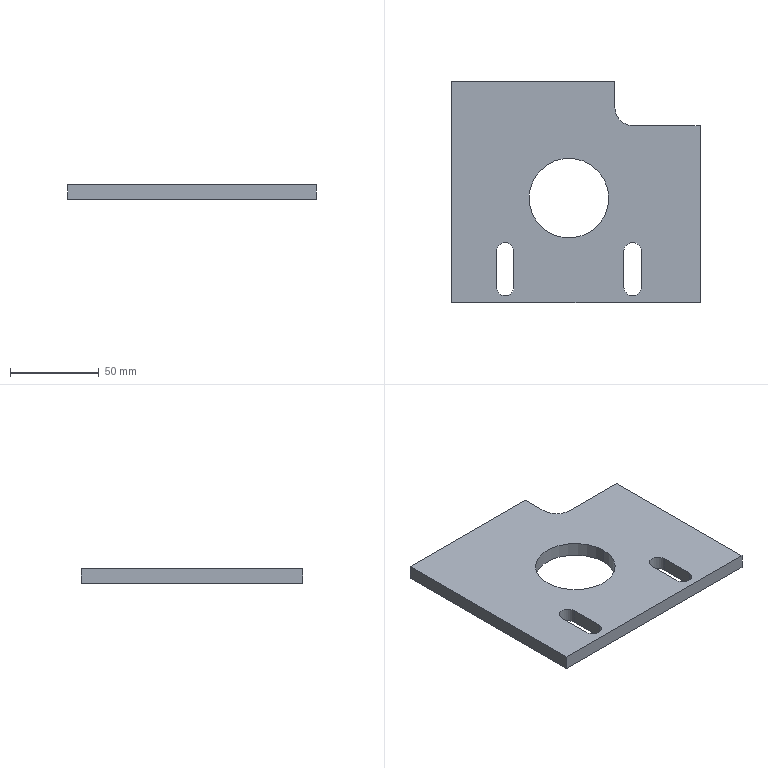Part | SolidWorks | features ICE 3, Extrusion 1, Fillet 1, LPattern 1 | 1 solid | 19 faces | box 140 x 125 x 8 mm | volume 113392 mm3 | plane 12 | cylinder 7 | commonest cylinder face diameters 10 x4 45 x2 20 x1
STEP:
#1=CARTESIAN_POINT('',(43.5,-66.,0.));
#2=VERTEX_POINT('',#1);
#3=CARTESIAN_POINT('',(88.5,-66.,0.));
#4=VERTEX_POINT('',#3);
#5=CARTESIAN_POINT('',(66.,-66.,0.));
#6=DIRECTION('',(0.,0.,1.));
#7=DIRECTION('',(1.,0.,0.));
#8=AXIS2_PLACEMENT_3D('',#5,#6,#7);
#9=CIRCLE('',#8,22.5);
#10=EDGE_CURVE('',#2,#4,#9,.T.);
#11=ORIENTED_EDGE('',*,*,#10,.F.);
#12=CARTESIAN_POINT('',(43.5,-66.,8.));
#13=VERTEX_POINT('',#12);
#14=CARTESIAN_POINT('',(43.5,-66.,0.));
#15=DIRECTION('',(0.,0.,1.));
#16=VECTOR('',#15,1000.);
#17=LINE('',#14,#16);
#18=EDGE_CURVE('',#2,#13,#17,.T.);
#19=ORIENTED_EDGE('',*,*,#18,.T.);
#20=CARTESIAN_POINT('',(88.5,-66.,8.));
#21=VERTEX_POINT('',#20);
#22=CARTESIAN_POINT('',(66.,-66.,8.));
#23=DIRECTION('',(0.,0.,1.));
#24=DIRECTION('',(1.,0.,0.));
#25=AXIS2_PLACEMENT_3D('',#22,#23,#24);
#26=CIRCLE('',#25,22.5);
#27=EDGE_CURVE('',#13,#21,#26,.T.);
#28=ORIENTED_EDGE('',*,*,#27,.T.);
#29=CARTESIAN_POINT('',(88.5,-66.,0.));
#30=DIRECTION('',(0.,0.,1.));
#31=VECTOR('',#30,1000.);
#32=LINE('',#29,#31);
#33=EDGE_CURVE('',#4,#21,#32,.T.);
#34=ORIENTED_EDGE('',*,*,#33,.F.);
#35=EDGE_LOOP('',(#11,#19,#28,#34));
#36=FACE_OUTER_BOUND('',#35,.T.);
#37=CARTESIAN_POINT('',(66.,-66.,0.));
#38=DIRECTION('',(0.,0.,1.));
#39=DIRECTION('',(1.,0.,0.));
#40=AXIS2_PLACEMENT_3D('',#37,#38,#39);
#41=CYLINDRICAL_SURFACE('',#40,22.5);
#42=ADVANCED_FACE('',(#36),#41,.F.);
#43=CARTESIAN_POINT('',(0.,0.,0.));
#44=VERTEX_POINT('',#43);
#45=CARTESIAN_POINT('',(0.,-125.,0.));
#46=VERTEX_POINT('',#45);
#47=CARTESIAN_POINT('',(0.,0.,0.));
#48=DIRECTION('',(0.,-1.,0.));
#49=VECTOR('',#48,1000.);
#50=LINE('',#47,#49);
#51=EDGE_CURVE('',#44,#46,#50,.T.);
#52=ORIENTED_EDGE('',*,*,#51,.T.);
#53=CARTESIAN_POINT('',(0.,-125.,8.));
#54=VERTEX_POINT('',#53);
#55=CARTESIAN_POINT('',(0.,-125.,8.));
#56=DIRECTION('',(0.,0.,-1.));
#57=VECTOR('',#56,1000.);
#58=LINE('',#55,#57);
#59=EDGE_CURVE('',#54,#46,#58,.T.);
#60=ORIENTED_EDGE('',*,*,#59,.F.);
#61=CARTESIAN_POINT('',(0.,0.,8.));
#62=VERTEX_POINT('',#61);
#63=CARTESIAN_POINT('',(0.,0.,8.));
#64=DIRECTION('',(0.,-1.,0.));
#65=VECTOR('',#64,1000.);
#66=LINE('',#63,#65);
#67=EDGE_CURVE('',#62,#54,#66,.T.);
#68=ORIENTED_EDGE('',*,*,#67,.F.);
#69=CARTESIAN_POINT('',(0.,0.,8.));
#70=DIRECTION('',(0.,0.,-1.));
#71=VECTOR('',#70,1000.);
#72=LINE('',#69,#71);
#73=EDGE_CURVE('',#62,#44,#72,.T.);
#74=ORIENTED_EDGE('',*,*,#73,.T.);
#75=EDGE_LOOP('',(#52,#60,#68,#74));
#76=FACE_OUTER_BOUND('',#75,.T.);
#77=CARTESIAN_POINT('',(0.,0.,8.));
#78=DIRECTION('',(1.,0.,0.));
#79=DIRECTION('',(0.,0.,-1.));
#80=AXIS2_PLACEMENT_3D('',#77,#78,#79);
#81=PLANE('',#80);
#82=ADVANCED_FACE('',(#76),#81,.F.);
#83=CARTESIAN_POINT('',(140.,-125.,0.));
#84=VERTEX_POINT('',#83);
#85=CARTESIAN_POINT('',(0.,-125.,0.));
#86=DIRECTION('',(1.,0.,0.));
#87=VECTOR('',#86,1000.);
#88=LINE('',#85,#87);
#89=EDGE_CURVE('',#46,#84,#88,.T.);
#90=ORIENTED_EDGE('',*,*,#89,.T.);
#91=CARTESIAN_POINT('',(140.,-125.,8.));
#92=VERTEX_POINT('',#91);
#93=CARTESIAN_POINT('',(140.,-125.,8.));
#94=DIRECTION('',(0.,0.,-1.));
#95=VECTOR('',#94,1000.);
#96=LINE('',#93,#95);
#97=EDGE_CURVE('',#92,#84,#96,.T.);
#98=ORIENTED_EDGE('',*,*,#97,.F.);
#99=CARTESIAN_POINT('',(0.,-125.,8.));
#100=DIRECTION('',(1.,0.,0.));
#101=VECTOR('',#100,1000.);
#102=LINE('',#99,#101);
#103=EDGE_CURVE('',#54,#92,#102,.T.);
#104=ORIENTED_EDGE('',*,*,#103,.F.);
#105=ORIENTED_EDGE('',*,*,#59,.T.);
#106=EDGE_LOOP('',(#90,#98,#104,#105));
#107=FACE_OUTER_BOUND('',#106,.T.);
#108=CARTESIAN_POINT('',(0.,-125.,8.));
#109=DIRECTION('',(0.,1.,0.));
#110=DIRECTION('',(0.,0.,1.));
#111=AXIS2_PLACEMENT_3D('',#108,#109,#110);
#112=PLANE('',#111);
#113=ADVANCED_FACE('',(#107),#112,.F.);
#114=CARTESIAN_POINT('',(140.,-25.,0.));
#115=VERTEX_POINT('',#114);
#116=CARTESIAN_POINT('',(140.,0.,0.));
#117=DIRECTION('',(0.,1.,0.));
#118=VECTOR('',#117,1000.);
#119=LINE('',#116,#118);
#120=EDGE_CURVE('',#84,#115,#119,.T.);
#121=ORIENTED_EDGE('',*,*,#120,.T.);
#122=CARTESIAN_POINT('',(140.,-25.,8.));
#123=VERTEX_POINT('',#122);
#124=CARTESIAN_POINT('',(140.,-25.,0.));
#125=DIRECTION('',(0.,0.,1.));
#126=VECTOR('',#125,1000.);
#127=LINE('',#124,#126);
#128=EDGE_CURVE('',#115,#123,#127,.T.);
#129=ORIENTED_EDGE('',*,*,#128,.T.);
#130=CARTESIAN_POINT('',(140.,0.,8.));
#131=DIRECTION('',(0.,1.,0.));
#132=VECTOR('',#131,1000.);
#133=LINE('',#130,#132);
#134=EDGE_CURVE('',#92,#123,#133,.T.);
#135=ORIENTED_EDGE('',*,*,#134,.F.);
#136=ORIENTED_EDGE('',*,*,#97,.T.);
#137=EDGE_LOOP('',(#121,#129,#135,#136));
#138=FACE_OUTER_BOUND('',#137,.T.);
#139=CARTESIAN_POINT('',(140.,0.,8.));
#140=DIRECTION('',(-1.,0.,0.));
#141=DIRECTION('',(0.,-1.,0.));
#142=AXIS2_PLACEMENT_3D('',#139,#140,#141);
#143=PLANE('',#142);
#144=ADVANCED_FACE('',(#138),#143,.F.);
#145=CARTESIAN_POINT('',(92.,0.,8.));
#146=VERTEX_POINT('',#145);
#147=CARTESIAN_POINT('',(0.,0.,8.));
#148=DIRECTION('',(-1.,0.,0.));
#149=VECTOR('',#148,1000.);
#150=LINE('',#147,#149);
#151=EDGE_CURVE('',#146,#62,#150,.T.);
#152=ORIENTED_EDGE('',*,*,#151,.F.);
#153=CARTESIAN_POINT('',(92.,0.,0.));
#154=VERTEX_POINT('',#153);
#155=CARTESIAN_POINT('',(92.,0.,0.));
#156=DIRECTION('',(0.,0.,1.));
#157=VECTOR('',#156,1000.);
#158=LINE('',#155,#157);
#159=EDGE_CURVE('',#154,#146,#158,.T.);
#160=ORIENTED_EDGE('',*,*,#159,.F.);
#161=CARTESIAN_POINT('',(0.,0.,0.));
#162=DIRECTION('',(-1.,0.,0.));
#163=VECTOR('',#162,1000.);
#164=LINE('',#161,#163);
#165=EDGE_CURVE('',#154,#44,#164,.T.);
#166=ORIENTED_EDGE('',*,*,#165,.T.);
#167=ORIENTED_EDGE('',*,*,#73,.F.);
#168=EDGE_LOOP('',(#152,#160,#166,#167));
#169=FACE_OUTER_BOUND('',#168,.T.);
#170=CARTESIAN_POINT('',(0.,0.,8.));
#171=DIRECTION('',(0.,-1.,0.));
#172=DIRECTION('',(0.,0.,-1.));
#173=AXIS2_PLACEMENT_3D('',#170,#171,#172);
#174=PLANE('',#173);
#175=ADVANCED_FACE('',(#169),#174,.F.);
#176=CARTESIAN_POINT('',(92.,-15.,8.));
#177=VERTEX_POINT('',#176);
#178=CARTESIAN_POINT('',(92.,0.,8.));
#179=DIRECTION('',(0.,-1.,0.));
#180=VECTOR('',#179,1000.);
#181=LINE('',#178,#180);
#182=EDGE_CURVE('',#146,#177,#181,.T.);
#183=ORIENTED_EDGE('',*,*,#182,.F.);
#184=ORIENTED_EDGE('',*,*,#151,.T.);
#185=ORIENTED_EDGE('',*,*,#67,.T.);
#186=ORIENTED_EDGE('',*,*,#103,.T.);
#187=ORIENTED_EDGE('',*,*,#134,.T.);
#188=CARTESIAN_POINT('',(102.,-25.,8.));
#189=VERTEX_POINT('',#188);
#190=CARTESIAN_POINT('',(92.,-25.,8.));
#191=DIRECTION('',(1.,0.,0.));
#192=VECTOR('',#191,1000.);
#193=LINE('',#190,#192);
#194=EDGE_CURVE('',#189,#123,#193,.T.);
#195=ORIENTED_EDGE('',*,*,#194,.F.);
#196=CARTESIAN_POINT('',(102.,-15.,8.));
#197=DIRECTION('',(0.,0.,-1.));
#198=DIRECTION('',(1.,0.,0.));
#199=AXIS2_PLACEMENT_3D('',#196,#197,#198);
#200=CIRCLE('',#199,10.);
#201=EDGE_CURVE('',#189,#177,#200,.T.);
#202=ORIENTED_EDGE('',*,*,#201,.T.);
#203=EDGE_LOOP('',(#183,#184,#185,#186,#187,#195,#202));
#204=FACE_OUTER_BOUND('',#203,.T.);
#205=CARTESIAN_POINT('',(107.,-96.,8.));
#206=VERTEX_POINT('',#205);
#207=CARTESIAN_POINT('',(97.,-96.,8.));
#208=VERTEX_POINT('',#207);
#209=CARTESIAN_POINT('',(102.,-96.,8.));
#210=DIRECTION('',(0.,0.,1.));
#211=DIRECTION('',(1.,0.,0.));
#212=AXIS2_PLACEMENT_3D('',#209,#210,#211);
#213=CIRCLE('',#212,5.);
#214=EDGE_CURVE('',#206,#208,#213,.T.);
#215=ORIENTED_EDGE('',*,*,#214,.F.);
#216=CARTESIAN_POINT('',(107.,-116.,8.));
#217=VERTEX_POINT('',#216);
#218=CARTESIAN_POINT('',(107.,-96.,8.));
#219=DIRECTION('',(0.,1.,0.));
#220=VECTOR('',#219,1000.);
#221=LINE('',#218,#220);
#222=EDGE_CURVE('',#217,#206,#221,.T.);
#223=ORIENTED_EDGE('',*,*,#222,.F.);
#224=CARTESIAN_POINT('',(97.,-116.,8.));
#225=VERTEX_POINT('',#224);
#226=CARTESIAN_POINT('',(102.,-116.,8.));
#227=DIRECTION('',(0.,0.,1.));
#228=DIRECTION('',(1.,0.,0.));
#229=AXIS2_PLACEMENT_3D('',#226,#227,#228);
#230=CIRCLE('',#229,5.);
#231=EDGE_CURVE('',#225,#217,#230,.T.);
#232=ORIENTED_EDGE('',*,*,#231,.F.);
#233=CARTESIAN_POINT('',(97.,-96.,8.));
#234=DIRECTION('',(0.,-1.,0.));
#235=VECTOR('',#234,1000.);
#236=LINE('',#233,#235);
#237=EDGE_CURVE('',#208,#225,#236,.T.);
#238=ORIENTED_EDGE('',*,*,#237,.F.);
#239=EDGE_LOOP('',(#215,#223,#232,#238));
#240=FACE_BOUND('',#239,.T.);
#241=CARTESIAN_POINT('',(35.,-96.,8.));
#242=VERTEX_POINT('',#241);
#243=CARTESIAN_POINT('',(25.,-96.,8.));
#244=VERTEX_POINT('',#243);
#245=CARTESIAN_POINT('',(30.,-96.,8.));
#246=DIRECTION('',(0.,0.,1.));
#247=DIRECTION('',(1.,0.,0.));
#248=AXIS2_PLACEMENT_3D('',#245,#246,#247);
#249=CIRCLE('',#248,5.);
#250=EDGE_CURVE('',#242,#244,#249,.T.);
#251=ORIENTED_EDGE('',*,*,#250,.F.);
#252=CARTESIAN_POINT('',(35.,-116.,8.));
#253=VERTEX_POINT('',#252);
#254=CARTESIAN_POINT('',(35.,-96.,8.));
#255=DIRECTION('',(0.,1.,0.));
#256=VECTOR('',#255,1000.);
#257=LINE('',#254,#256);
#258=EDGE_CURVE('',#253,#242,#257,.T.);
#259=ORIENTED_EDGE('',*,*,#258,.F.);
#260=CARTESIAN_POINT('',(25.,-116.,8.));
#261=VERTEX_POINT('',#260);
#262=CARTESIAN_POINT('',(30.,-116.,8.));
#263=DIRECTION('',(0.,0.,1.));
#264=DIRECTION('',(1.,0.,0.));
#265=AXIS2_PLACEMENT_3D('',#262,#263,#264);
#266=CIRCLE('',#265,5.);
#267=EDGE_CURVE('',#261,#253,#266,.T.);
#268=ORIENTED_EDGE('',*,*,#267,.F.);
#269=CARTESIAN_POINT('',(25.,-96.,8.));
#270=DIRECTION('',(0.,-1.,0.));
#271=VECTOR('',#270,1000.);
#272=LINE('',#269,#271);
#273=EDGE_CURVE('',#244,#261,#272,.T.);
#274=ORIENTED_EDGE('',*,*,#273,.F.);
#275=EDGE_LOOP('',(#251,#259,#268,#274));
#276=FACE_BOUND('',#275,.T.);
#277=CARTESIAN_POINT('',(66.,-66.,8.));
#278=DIRECTION('',(0.,0.,1.));
#279=DIRECTION('',(1.,0.,0.));
#280=AXIS2_PLACEMENT_3D('',#277,#278,#279);
#281=CIRCLE('',#280,22.5);
#282=EDGE_CURVE('',#21,#13,#281,.T.);
#283=ORIENTED_EDGE('',*,*,#282,.F.);
#284=ORIENTED_EDGE('',*,*,#27,.F.);
#285=EDGE_LOOP('',(#283,#284));
#286=FACE_BOUND('',#285,.T.);
#287=CARTESIAN_POINT('',(0.,0.,8.));
#288=DIRECTION('',(0.,0.,1.));
#289=DIRECTION('',(1.,0.,0.));
#290=AXIS2_PLACEMENT_3D('',#287,#288,#289);
#291=PLANE('',#290);
#292=ADVANCED_FACE('',(#204,#240,#276,#286),#291,.T.);
#293=CARTESIAN_POINT('',(107.,-116.,0.));
#294=VERTEX_POINT('',#293);
#295=CARTESIAN_POINT('',(107.,-96.,0.));
#296=VERTEX_POINT('',#295);
#297=CARTESIAN_POINT('',(107.,-96.,0.));
#298=DIRECTION('',(0.,1.,0.));
#299=VECTOR('',#298,1000.);
#300=LINE('',#297,#299);
#301=EDGE_CURVE('',#294,#296,#300,.T.);
#302=ORIENTED_EDGE('',*,*,#301,.T.);
#303=CARTESIAN_POINT('',(97.,-96.,0.));
#304=VERTEX_POINT('',#303);
#305=CARTESIAN_POINT('',(102.,-96.,0.));
#306=DIRECTION('',(0.,0.,1.));
#307=DIRECTION('',(1.,0.,0.));
#308=AXIS2_PLACEMENT_3D('',#305,#306,#307);
#309=CIRCLE('',#308,5.);
#310=EDGE_CURVE('',#296,#304,#309,.T.);
#311=ORIENTED_EDGE('',*,*,#310,.T.);
#312=CARTESIAN_POINT('',(97.,-116.,0.));
#313=VERTEX_POINT('',#312);
#314=CARTESIAN_POINT('',(97.,-96.,0.));
#315=DIRECTION('',(0.,-1.,0.));
#316=VECTOR('',#315,1000.);
#317=LINE('',#314,#316);
#318=EDGE_CURVE('',#304,#313,#317,.T.);
#319=ORIENTED_EDGE('',*,*,#318,.T.);
#320=CARTESIAN_POINT('',(102.,-116.,0.));
#321=DIRECTION('',(0.,0.,1.));
#322=DIRECTION('',(1.,0.,0.));
#323=AXIS2_PLACEMENT_3D('',#320,#321,#322);
#324=CIRCLE('',#323,5.);
#325=EDGE_CURVE('',#313,#294,#324,.T.);
#326=ORIENTED_EDGE('',*,*,#325,.T.);
#327=EDGE_LOOP('',(#302,#311,#319,#326));
#328=FACE_BOUND('',#327,.T.);
#329=CARTESIAN_POINT('',(35.,-116.,0.));
#330=VERTEX_POINT('',#329);
#331=CARTESIAN_POINT('',(35.,-96.,0.));
#332=VERTEX_POINT('',#331);
#333=CARTESIAN_POINT('',(35.,-96.,0.));
#334=DIRECTION('',(0.,1.,0.));
#335=VECTOR('',#334,1000.);
#336=LINE('',#333,#335);
#337=EDGE_CURVE('',#330,#332,#336,.T.);
#338=ORIENTED_EDGE('',*,*,#337,.T.);
#339=CARTESIAN_POINT('',(25.,-96.,0.));
#340=VERTEX_POINT('',#339);
#341=CARTESIAN_POINT('',(30.,-96.,0.));
#342=DIRECTION('',(0.,0.,1.));
#343=DIRECTION('',(1.,0.,0.));
#344=AXIS2_PLACEMENT_3D('',#341,#342,#343);
#345=CIRCLE('',#344,5.);
#346=EDGE_CURVE('',#332,#340,#345,.T.);
#347=ORIENTED_EDGE('',*,*,#346,.T.);
#348=CARTESIAN_POINT('',(25.,-116.,0.));
#349=VERTEX_POINT('',#348);
#350=CARTESIAN_POINT('',(25.,-96.,0.));
#351=DIRECTION('',(0.,-1.,0.));
#352=VECTOR('',#351,1000.);
#353=LINE('',#350,#352);
#354=EDGE_CURVE('',#340,#349,#353,.T.);
#355=ORIENTED_EDGE('',*,*,#354,.T.);
#356=CARTESIAN_POINT('',(30.,-116.,0.));
#357=DIRECTION('',(0.,0.,1.));
#358=DIRECTION('',(1.,0.,0.));
#359=AXIS2_PLACEMENT_3D('',#356,#357,#358);
#360=CIRCLE('',#359,5.);
#361=EDGE_CURVE('',#349,#330,#360,.T.);
#362=ORIENTED_EDGE('',*,*,#361,.T.);
#363=EDGE_LOOP('',(#338,#347,#355,#362));
#364=FACE_BOUND('',#363,.T.);
#365=CARTESIAN_POINT('',(66.,-66.,0.));
#366=DIRECTION('',(0.,0.,1.));
#367=DIRECTION('',(1.,0.,0.));
#368=AXIS2_PLACEMENT_3D('',#365,#366,#367);
#369=CIRCLE('',#368,22.5);
#370=EDGE_CURVE('',#4,#2,#369,.T.);
#371=ORIENTED_EDGE('',*,*,#370,.T.);
#372=ORIENTED_EDGE('',*,*,#10,.T.);
#373=EDGE_LOOP('',(#371,#372));
#374=FACE_BOUND('',#373,.T.);
#375=ORIENTED_EDGE('',*,*,#165,.F.);
#376=CARTESIAN_POINT('',(92.,-15.,0.));
#377=VERTEX_POINT('',#376);
#378=CARTESIAN_POINT('',(92.,0.,0.));
#379=DIRECTION('',(0.,-1.,0.));
#380=VECTOR('',#379,1000.);
#381=LINE('',#378,#380);
#382=EDGE_CURVE('',#154,#377,#381,.T.);
#383=ORIENTED_EDGE('',*,*,#382,.T.);
#384=CARTESIAN_POINT('',(102.,-25.,0.));
#385=VERTEX_POINT('',#384);
#386=CARTESIAN_POINT('',(102.,-15.,0.));
#387=DIRECTION('',(0.,0.,1.));
#388=DIRECTION('',(1.,0.,0.));
#389=AXIS2_PLACEMENT_3D('',#386,#387,#388);
#390=CIRCLE('',#389,10.);
#391=EDGE_CURVE('',#377,#385,#390,.T.);
#392=ORIENTED_EDGE('',*,*,#391,.T.);
#393=CARTESIAN_POINT('',(92.,-25.,0.));
#394=DIRECTION('',(1.,0.,0.));
#395=VECTOR('',#394,1000.);
#396=LINE('',#393,#395);
#397=EDGE_CURVE('',#385,#115,#396,.T.);
#398=ORIENTED_EDGE('',*,*,#397,.T.);
#399=ORIENTED_EDGE('',*,*,#120,.F.);
#400=ORIENTED_EDGE('',*,*,#89,.F.);
#401=ORIENTED_EDGE('',*,*,#51,.F.);
#402=EDGE_LOOP('',(#375,#383,#392,#398,#399,#400,#401));
#403=FACE_OUTER_BOUND('',#402,.T.);
#404=CARTESIAN_POINT('',(0.,0.,0.));
#405=DIRECTION('',(0.,0.,1.));
#406=DIRECTION('',(1.,0.,0.));
#407=AXIS2_PLACEMENT_3D('',#404,#405,#406);
#408=PLANE('',#407);
#409=ADVANCED_FACE('',(#328,#364,#374,#403),#408,.F.);
#410=ORIENTED_EDGE('',*,*,#18,.F.);
#411=ORIENTED_EDGE('',*,*,#370,.F.);
#412=ORIENTED_EDGE('',*,*,#33,.T.);
#413=ORIENTED_EDGE('',*,*,#282,.T.);
#414=EDGE_LOOP('',(#410,#411,#412,#413));
#415=FACE_OUTER_BOUND('',#414,.T.);
#416=CARTESIAN_POINT('',(66.,-66.,0.));
#417=DIRECTION('',(0.,0.,1.));
#418=DIRECTION('',(1.,0.,0.));
#419=AXIS2_PLACEMENT_3D('',#416,#417,#418);
#420=CYLINDRICAL_SURFACE('',#419,22.5);
#421=ADVANCED_FACE('',(#415),#420,.F.);
#422=ORIENTED_EDGE('',*,*,#250,.T.);
#423=CARTESIAN_POINT('',(25.,-96.,0.));
#424=DIRECTION('',(0.,0.,1.));
#425=VECTOR('',#424,1000.);
#426=LINE('',#423,#425);
#427=EDGE_CURVE('',#340,#244,#426,.T.);
#428=ORIENTED_EDGE('',*,*,#427,.F.);
#429=ORIENTED_EDGE('',*,*,#346,.F.);
#430=CARTESIAN_POINT('',(35.,-96.,0.));
#431=DIRECTION('',(0.,0.,1.));
#432=VECTOR('',#431,1000.);
#433=LINE('',#430,#432);
#434=EDGE_CURVE('',#332,#242,#433,.T.);
#435=ORIENTED_EDGE('',*,*,#434,.T.);
#436=EDGE_LOOP('',(#422,#428,#429,#435));
#437=FACE_OUTER_BOUND('',#436,.T.);
#438=CARTESIAN_POINT('',(30.,-96.,0.));
#439=DIRECTION('',(0.,0.,1.));
#440=DIRECTION('',(1.,0.,0.));
#441=AXIS2_PLACEMENT_3D('',#438,#439,#440);
#442=CYLINDRICAL_SURFACE('',#441,5.);
#443=ADVANCED_FACE('',(#437),#442,.F.);
#444=ORIENTED_EDGE('',*,*,#258,.T.);
#445=ORIENTED_EDGE('',*,*,#434,.F.);
#446=ORIENTED_EDGE('',*,*,#337,.F.);
#447=CARTESIAN_POINT('',(35.,-116.,0.));
#448=DIRECTION('',(0.,0.,1.));
#449=VECTOR('',#448,1000.);
#450=LINE('',#447,#449);
#451=EDGE_CURVE('',#330,#253,#450,.T.);
#452=ORIENTED_EDGE('',*,*,#451,.T.);
#453=EDGE_LOOP('',(#444,#445,#446,#452));
#454=FACE_OUTER_BOUND('',#453,.T.);
#455=CARTESIAN_POINT('',(35.,-96.,0.));
#456=DIRECTION('',(1.,0.,0.));
#457=DIRECTION('',(0.,1.,0.));
#458=AXIS2_PLACEMENT_3D('',#455,#456,#457);
#459=PLANE('',#458);
#460=ADVANCED_FACE('',(#454),#459,.F.);
#461=ORIENTED_EDGE('',*,*,#267,.T.);
#462=ORIENTED_EDGE('',*,*,#451,.F.);
#463=ORIENTED_EDGE('',*,*,#361,.F.);
#464=CARTESIAN_POINT('',(25.,-116.,0.));
#465=DIRECTION('',(0.,0.,1.));
#466=VECTOR('',#465,1000.);
#467=LINE('',#464,#466);
#468=EDGE_CURVE('',#349,#261,#467,.T.);
#469=ORIENTED_EDGE('',*,*,#468,.T.);
#470=EDGE_LOOP('',(#461,#462,#463,#469));
#471=FACE_OUTER_BOUND('',#470,.T.);
#472=CARTESIAN_POINT('',(30.,-116.,0.));
#473=DIRECTION('',(0.,0.,1.));
#474=DIRECTION('',(1.,0.,0.));
#475=AXIS2_PLACEMENT_3D('',#472,#473,#474);
#476=CYLINDRICAL_SURFACE('',#475,5.);
#477=ADVANCED_FACE('',(#471),#476,.F.);
#478=ORIENTED_EDGE('',*,*,#273,.T.);
#479=ORIENTED_EDGE('',*,*,#468,.F.);
#480=ORIENTED_EDGE('',*,*,#354,.F.);
#481=ORIENTED_EDGE('',*,*,#427,.T.);
#482=EDGE_LOOP('',(#478,#479,#480,#481));
#483=FACE_OUTER_BOUND('',#482,.T.);
#484=CARTESIAN_POINT('',(25.,-96.,0.));
#485=DIRECTION('',(-1.,0.,0.));
#486=DIRECTION('',(0.,-1.,0.));
#487=AXIS2_PLACEMENT_3D('',#484,#485,#486);
#488=PLANE('',#487);
#489=ADVANCED_FACE('',(#483),#488,.F.);
#490=ORIENTED_EDGE('',*,*,#214,.T.);
#491=CARTESIAN_POINT('',(97.,-96.,0.));
#492=DIRECTION('',(0.,0.,1.));
#493=VECTOR('',#492,1000.);
#494=LINE('',#491,#493);
#495=EDGE_CURVE('',#304,#208,#494,.T.);
#496=ORIENTED_EDGE('',*,*,#495,.F.);
#497=ORIENTED_EDGE('',*,*,#310,.F.);
#498=CARTESIAN_POINT('',(107.,-96.,0.));
#499=DIRECTION('',(0.,0.,1.));
#500=VECTOR('',#499,1000.);
#501=LINE('',#498,#500);
#502=EDGE_CURVE('',#296,#206,#501,.T.);
#503=ORIENTED_EDGE('',*,*,#502,.T.);
#504=EDGE_LOOP('',(#490,#496,#497,#503));
#505=FACE_OUTER_BOUND('',#504,.T.);
#506=CARTESIAN_POINT('',(102.,-96.,0.));
#507=DIRECTION('',(0.,0.,1.));
#508=DIRECTION('',(1.,0.,0.));
#509=AXIS2_PLACEMENT_3D('',#506,#507,#508);
#510=CYLINDRICAL_SURFACE('',#509,5.);
#511=ADVANCED_FACE('',(#505),#510,.F.);
#512=ORIENTED_EDGE('',*,*,#222,.T.);
#513=ORIENTED_EDGE('',*,*,#502,.F.);
#514=ORIENTED_EDGE('',*,*,#301,.F.);
#515=CARTESIAN_POINT('',(107.,-116.,0.));
#516=DIRECTION('',(0.,0.,1.));
#517=VECTOR('',#516,1000.);
#518=LINE('',#515,#517);
#519=EDGE_CURVE('',#294,#217,#518,.T.);
#520=ORIENTED_EDGE('',*,*,#519,.T.);
#521=EDGE_LOOP('',(#512,#513,#514,#520));
#522=FACE_OUTER_BOUND('',#521,.T.);
#523=CARTESIAN_POINT('',(107.,-96.,0.));
#524=DIRECTION('',(1.,0.,0.));
#525=DIRECTION('',(0.,1.,0.));
#526=AXIS2_PLACEMENT_3D('',#523,#524,#525);
#527=PLANE('',#526);
#528=ADVANCED_FACE('',(#522),#527,.F.);
#529=ORIENTED_EDGE('',*,*,#231,.T.);
#530=ORIENTED_EDGE('',*,*,#519,.F.);
#531=ORIENTED_EDGE('',*,*,#325,.F.);
#532=CARTESIAN_POINT('',(97.,-116.,0.));
#533=DIRECTION('',(0.,0.,1.));
#534=VECTOR('',#533,1000.);
#535=LINE('',#532,#534);
#536=EDGE_CURVE('',#313,#225,#535,.T.);
#537=ORIENTED_EDGE('',*,*,#536,.T.);
#538=EDGE_LOOP('',(#529,#530,#531,#537));
#539=FACE_OUTER_BOUND('',#538,.T.);
#540=CARTESIAN_POINT('',(102.,-116.,0.));
#541=DIRECTION('',(0.,0.,1.));
#542=DIRECTION('',(1.,0.,0.));
#543=AXIS2_PLACEMENT_3D('',#540,#541,#542);
#544=CYLINDRICAL_SURFACE('',#543,5.);
#545=ADVANCED_FACE('',(#539),#544,.F.);
#546=ORIENTED_EDGE('',*,*,#237,.T.);
#547=ORIENTED_EDGE('',*,*,#536,.F.);
#548=ORIENTED_EDGE('',*,*,#318,.F.);
#549=ORIENTED_EDGE('',*,*,#495,.T.);
#550=EDGE_LOOP('',(#546,#547,#548,#549));
#551=FACE_OUTER_BOUND('',#550,.T.);
#552=CARTESIAN_POINT('',(97.,-96.,0.));
#553=DIRECTION('',(-1.,0.,0.));
#554=DIRECTION('',(0.,-1.,0.));
#555=AXIS2_PLACEMENT_3D('',#552,#553,#554);
#556=PLANE('',#555);
#557=ADVANCED_FACE('',(#551),#556,.F.);
#558=ORIENTED_EDGE('',*,*,#182,.T.);
#559=CARTESIAN_POINT('',(92.,-15.,0.));
#560=DIRECTION('',(0.,0.,-1.));
#561=VECTOR('',#560,1000.);
#562=LINE('',#559,#561);
#563=EDGE_CURVE('',#177,#377,#562,.T.);
#564=ORIENTED_EDGE('',*,*,#563,.T.);
#565=ORIENTED_EDGE('',*,*,#382,.F.);
#566=ORIENTED_EDGE('',*,*,#159,.T.);
#567=EDGE_LOOP('',(#558,#564,#565,#566));
#568=FACE_OUTER_BOUND('',#567,.T.);
#569=CARTESIAN_POINT('',(92.,0.,0.));
#570=DIRECTION('',(-1.,0.,0.));
#571=DIRECTION('',(0.,0.,1.));
#572=AXIS2_PLACEMENT_3D('',#569,#570,#571);
#573=PLANE('',#572);
#574=ADVANCED_FACE('',(#568),#573,.F.);
#575=ORIENTED_EDGE('',*,*,#397,.F.);
#576=CARTESIAN_POINT('',(102.,-25.,8.));
#577=DIRECTION('',(0.,0.,1.));
#578=VECTOR('',#577,1000.);
#579=LINE('',#576,#578);
#580=EDGE_CURVE('',#385,#189,#579,.T.);
#581=ORIENTED_EDGE('',*,*,#580,.T.);
#582=ORIENTED_EDGE('',*,*,#194,.T.);
#583=ORIENTED_EDGE('',*,*,#128,.F.);
#584=EDGE_LOOP('',(#575,#581,#582,#583));
#585=FACE_OUTER_BOUND('',#584,.T.);
#586=CARTESIAN_POINT('',(92.,-25.,0.));
#587=DIRECTION('',(0.,-1.,0.));
#588=DIRECTION('',(0.,0.,-1.));
#589=AXIS2_PLACEMENT_3D('',#586,#587,#588);
#590=PLANE('',#589);
#591=ADVANCED_FACE('',(#585),#590,.F.);
#592=ORIENTED_EDGE('',*,*,#391,.F.);
#593=ORIENTED_EDGE('',*,*,#563,.F.);
#594=ORIENTED_EDGE('',*,*,#201,.F.);
#595=ORIENTED_EDGE('',*,*,#580,.F.);
#596=EDGE_LOOP('',(#592,#593,#594,#595));
#597=FACE_OUTER_BOUND('',#596,.T.);
#598=CARTESIAN_POINT('',(102.,-15.,0.));
#599=DIRECTION('',(0.,0.,-1.));
#600=DIRECTION('',(-1.,0.,0.));
#601=AXIS2_PLACEMENT_3D('',#598,#599,#600);
#602=CYLINDRICAL_SURFACE('',#601,10.);
#603=ADVANCED_FACE('',(#597),#602,.F.);
#604=CLOSED_SHELL('',(#42,#82,#113,#144,#175,#292,#409,#421,#443,#460,#477,#489,#511,#528,#545,#557,#574,#591,#603));
#605=MANIFOLD_SOLID_BREP('',#604);
#606=CARTESIAN_POINT('',(0.,0.,0.));
#607=DIRECTION('',(0.,0.,1.));
#608=DIRECTION('',(1.,0.,0.));
#609=AXIS2_PLACEMENT_3D('',#606,#607,#608);
#610=(LENGTH_UNIT()NAMED_UNIT(*)SI_UNIT(.MILLI.,.METRE.));
#611=UNCERTAINTY_MEASURE_WITH_UNIT(LENGTH_MEASURE(0.00001),#610,'','');
#612=(NAMED_UNIT(*)PLANE_ANGLE_UNIT()SI_UNIT($,.RADIAN.));
#613=(NAMED_UNIT(*)SI_UNIT($,.STERADIAN.)SOLID_ANGLE_UNIT());
#614=(GEOMETRIC_REPRESENTATION_CONTEXT(3)GLOBAL_UNCERTAINTY_ASSIGNED_CONTEXT((#611))GLOBAL_UNIT_ASSIGNED_CONTEXT((#610,#612,#613))REPRESENTATION_CONTEXT('',''));
#615=ADVANCED_BREP_SHAPE_REPRESENTATION('',(#605,#609),#614);